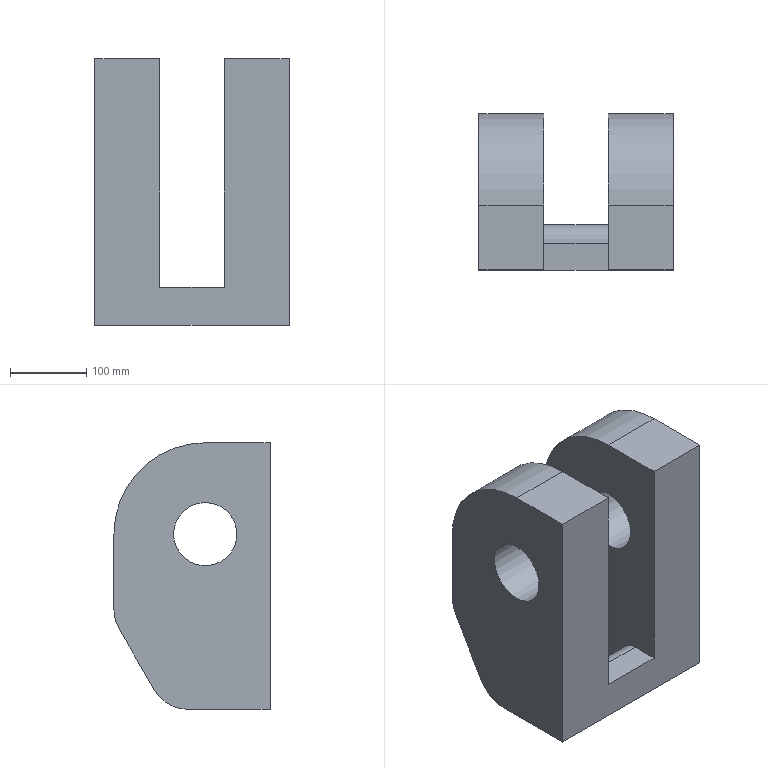Part | NX | features solid 2 | 1 solid | 22 faces | box 255 x 205 x 350 mm | volume 10284729 mm3 | plane 13 | cylinder 9 | commonest cylinder face diameters 100 x4 83 x2 240 x2 50 x1
STEP:
#1=CARTESIAN_POINT('',(-1395.,1008.453,-630.));
#2=VERTEX_POINT('',#1);
#3=CARTESIAN_POINT('',(-1395.,935.,-630.));
#4=VERTEX_POINT('',#3);
#5=CARTESIAN_POINT('',(-1395.,1105.,-630.));
#6=DIRECTION('',(0.,-1.,0.));
#7=VECTOR('',#6,1000.);
#8=LINE('',#5,#7);
#9=EDGE_CURVE('',#2,#4,#8,.T.);
#10=ORIENTED_EDGE('',*,*,#9,.F.);
#11=CARTESIAN_POINT('',(-1310.,1008.453,-630.));
#12=VERTEX_POINT('',#11);
#13=CARTESIAN_POINT('',(-1310.,1008.453,-630.));
#14=DIRECTION('',(1.,0.,0.));
#15=VECTOR('',#14,1000.);
#16=LINE('',#13,#15);
#17=EDGE_CURVE('',#2,#12,#16,.T.);
#18=ORIENTED_EDGE('',*,*,#17,.T.);
#19=CARTESIAN_POINT('',(-1310.,900.,-630.));
#20=VERTEX_POINT('',#19);
#21=CARTESIAN_POINT('',(-1310.,1105.,-630.));
#22=DIRECTION('',(0.,-1.,0.));
#23=VECTOR('',#22,1000.);
#24=LINE('',#21,#23);
#25=EDGE_CURVE('',#12,#20,#24,.T.);
#26=ORIENTED_EDGE('',*,*,#25,.T.);
#27=CARTESIAN_POINT('',(-1565.,900.,-630.));
#28=VERTEX_POINT('',#27);
#29=CARTESIAN_POINT('',(-1565.,900.,-630.));
#30=DIRECTION('',(1.,0.,0.));
#31=VECTOR('',#30,1000.);
#32=LINE('',#29,#31);
#33=EDGE_CURVE('',#28,#20,#32,.T.);
#34=ORIENTED_EDGE('',*,*,#33,.F.);
#35=CARTESIAN_POINT('',(-1565.,1008.453,-630.));
#36=VERTEX_POINT('',#35);
#37=CARTESIAN_POINT('',(-1565.,1105.,-630.));
#38=DIRECTION('',(0.,-1.,0.));
#39=VECTOR('',#38,1000.);
#40=LINE('',#37,#39);
#41=EDGE_CURVE('',#36,#28,#40,.T.);
#42=ORIENTED_EDGE('',*,*,#41,.F.);
#43=CARTESIAN_POINT('',(-1480.,1008.453,-630.));
#44=VERTEX_POINT('',#43);
#45=CARTESIAN_POINT('',(-1480.,1008.453,-630.));
#46=DIRECTION('',(1.,0.,0.));
#47=VECTOR('',#46,1000.);
#48=LINE('',#45,#47);
#49=EDGE_CURVE('',#36,#44,#48,.T.);
#50=ORIENTED_EDGE('',*,*,#49,.T.);
#51=CARTESIAN_POINT('',(-1480.,935.,-630.));
#52=VERTEX_POINT('',#51);
#53=CARTESIAN_POINT('',(-1480.,1105.,-630.));
#54=DIRECTION('',(0.,-1.,0.));
#55=VECTOR('',#54,1000.);
#56=LINE('',#53,#55);
#57=EDGE_CURVE('',#44,#52,#56,.T.);
#58=ORIENTED_EDGE('',*,*,#57,.T.);
#59=CARTESIAN_POINT('',(-1437.5,935.,-630.));
#60=DIRECTION('',(1.,0.,0.));
#61=VECTOR('',#60,1000.);
#62=LINE('',#59,#61);
#63=EDGE_CURVE('',#4,#52,#62,.F.);
#64=ORIENTED_EDGE('',*,*,#63,.F.);
#65=EDGE_LOOP('',(#10,#18,#26,#34,#42,#50,#58,#64));
#66=FACE_BOUND('',#65,.T.);
#67=CARTESIAN_POINT('',(-1565.,1105.,-630.));
#68=DIRECTION('',(0.,0.,1.));
#69=DIRECTION('',(0.,-1.,0.));
#70=AXIS2_PLACEMENT_3D('',#67,#68,#69);
#71=PLANE('',#70);
#72=ADVANCED_FACE('',(#66),#71,.F.);
#73=CARTESIAN_POINT('',(-1565.,985.,-280.));
#74=VERTEX_POINT('',#73);
#75=CARTESIAN_POINT('',(-1565.,900.,-280.));
#76=VERTEX_POINT('',#75);
#77=CARTESIAN_POINT('',(-1565.,1105.,-280.));
#78=DIRECTION('',(0.,-1.,0.));
#79=VECTOR('',#78,1000.);
#80=LINE('',#77,#79);
#81=EDGE_CURVE('',#74,#76,#80,.T.);
#82=ORIENTED_EDGE('',*,*,#81,.T.);
#83=CARTESIAN_POINT('',(-1480.,900.,-280.));
#84=VERTEX_POINT('',#83);
#85=CARTESIAN_POINT('',(-1565.,900.,-280.));
#86=DIRECTION('',(1.,0.,0.));
#87=VECTOR('',#86,1000.);
#88=LINE('',#85,#87);
#89=EDGE_CURVE('',#76,#84,#88,.T.);
#90=ORIENTED_EDGE('',*,*,#89,.T.);
#91=CARTESIAN_POINT('',(-1480.,985.,-280.));
#92=VERTEX_POINT('',#91);
#93=CARTESIAN_POINT('',(-1480.,1105.,-280.));
#94=DIRECTION('',(0.,1.,0.));
#95=VECTOR('',#94,1000.);
#96=LINE('',#93,#95);
#97=EDGE_CURVE('',#92,#84,#96,.F.);
#98=ORIENTED_EDGE('',*,*,#97,.F.);
#99=CARTESIAN_POINT('',(-1565.,985.,-280.));
#100=DIRECTION('',(-1.,0.,0.));
#101=VECTOR('',#100,1000.);
#102=LINE('',#99,#101);
#103=EDGE_CURVE('',#74,#92,#102,.F.);
#104=ORIENTED_EDGE('',*,*,#103,.F.);
#105=EDGE_LOOP('',(#82,#90,#98,#104));
#106=FACE_BOUND('',#105,.T.);
#107=CARTESIAN_POINT('',(-1565.,1105.,-280.));
#108=DIRECTION('',(0.,0.,1.));
#109=DIRECTION('',(0.,-1.,0.));
#110=AXIS2_PLACEMENT_3D('',#107,#108,#109);
#111=PLANE('',#110);
#112=ADVANCED_FACE('',(#106),#111,.T.);
#113=CARTESIAN_POINT('',(-1480.,1105.,-400.));
#114=VERTEX_POINT('',#113);
#115=CARTESIAN_POINT('',(-1480.,1105.,-499.378));
#116=VERTEX_POINT('',#115);
#117=CARTESIAN_POINT('',(-1480.,1105.,-280.));
#118=DIRECTION('',(0.,0.,-1.));
#119=VECTOR('',#118,1000.);
#120=LINE('',#117,#119);
#121=EDGE_CURVE('',#114,#116,#120,.T.);
#122=ORIENTED_EDGE('',*,*,#121,.T.);
#123=CARTESIAN_POINT('',(-1565.,1105.,-499.378));
#124=VERTEX_POINT('',#123);
#125=CARTESIAN_POINT('',(-1565.,1105.,-499.378));
#126=DIRECTION('',(-1.,0.,0.));
#127=VECTOR('',#126,1000.);
#128=LINE('',#125,#127);
#129=EDGE_CURVE('',#116,#124,#128,.T.);
#130=ORIENTED_EDGE('',*,*,#129,.T.);
#131=CARTESIAN_POINT('',(-1565.,1105.,-400.));
#132=VERTEX_POINT('',#131);
#133=CARTESIAN_POINT('',(-1565.,1105.,-280.));
#134=DIRECTION('',(0.,0.,-1.));
#135=VECTOR('',#134,1000.);
#136=LINE('',#133,#135);
#137=EDGE_CURVE('',#132,#124,#136,.T.);
#138=ORIENTED_EDGE('',*,*,#137,.F.);
#139=CARTESIAN_POINT('',(-1565.,1105.,-400.));
#140=DIRECTION('',(1.,0.,0.));
#141=VECTOR('',#140,1000.);
#142=LINE('',#139,#141);
#143=EDGE_CURVE('',#114,#132,#142,.F.);
#144=ORIENTED_EDGE('',*,*,#143,.F.);
#145=EDGE_LOOP('',(#122,#130,#138,#144));
#146=FACE_BOUND('',#145,.T.);
#147=CARTESIAN_POINT('',(-1565.,1105.,-280.));
#148=DIRECTION('',(0.,-1.,0.));
#149=DIRECTION('',(0.,0.,-1.));
#150=AXIS2_PLACEMENT_3D('',#147,#148,#149);
#151=PLANE('',#150);
#152=ADVANCED_FACE('',(#146),#151,.F.);
#153=CARTESIAN_POINT('',(-1310.,900.,-280.));
#154=VERTEX_POINT('',#153);
#155=CARTESIAN_POINT('',(-1310.,900.,-245.));
#156=DIRECTION('',(0.,0.,-1.));
#157=VECTOR('',#156,1000.);
#158=LINE('',#155,#157);
#159=EDGE_CURVE('',#154,#20,#158,.T.);
#160=ORIENTED_EDGE('',*,*,#159,.F.);
#161=CARTESIAN_POINT('',(-1395.,900.,-280.));
#162=VERTEX_POINT('',#161);
#163=CARTESIAN_POINT('',(-1395.,900.,-280.));
#164=DIRECTION('',(1.,0.,0.));
#165=VECTOR('',#164,1000.);
#166=LINE('',#163,#165);
#167=EDGE_CURVE('',#162,#154,#166,.T.);
#168=ORIENTED_EDGE('',*,*,#167,.F.);
#169=CARTESIAN_POINT('',(-1395.,900.,-580.));
#170=VERTEX_POINT('',#169);
#171=CARTESIAN_POINT('',(-1395.,900.,-245.));
#172=DIRECTION('',(0.,0.,-1.));
#173=VECTOR('',#172,1000.);
#174=LINE('',#171,#173);
#175=EDGE_CURVE('',#162,#170,#174,.T.);
#176=ORIENTED_EDGE('',*,*,#175,.T.);
#177=CARTESIAN_POINT('',(-1480.,900.,-580.));
#178=VERTEX_POINT('',#177);
#179=CARTESIAN_POINT('',(-1437.5,900.,-580.));
#180=DIRECTION('',(1.,0.,0.));
#181=VECTOR('',#180,1000.);
#182=LINE('',#179,#181);
#183=EDGE_CURVE('',#178,#170,#182,.T.);
#184=ORIENTED_EDGE('',*,*,#183,.F.);
#185=CARTESIAN_POINT('',(-1480.,900.,-245.));
#186=DIRECTION('',(0.,0.,-1.));
#187=VECTOR('',#186,1000.);
#188=LINE('',#185,#187);
#189=EDGE_CURVE('',#84,#178,#188,.T.);
#190=ORIENTED_EDGE('',*,*,#189,.F.);
#191=ORIENTED_EDGE('',*,*,#89,.F.);
#192=CARTESIAN_POINT('',(-1565.,900.,-245.));
#193=DIRECTION('',(0.,0.,-1.));
#194=VECTOR('',#193,1000.);
#195=LINE('',#192,#194);
#196=EDGE_CURVE('',#76,#28,#195,.T.);
#197=ORIENTED_EDGE('',*,*,#196,.T.);
#198=ORIENTED_EDGE('',*,*,#33,.T.);
#199=EDGE_LOOP('',(#160,#168,#176,#184,#190,#191,#197,#198));
#200=FACE_BOUND('',#199,.T.);
#201=CARTESIAN_POINT('',(-1565.,900.,-245.));
#202=DIRECTION('',(0.,-1.,0.));
#203=DIRECTION('',(0.,0.,-1.));
#204=AXIS2_PLACEMENT_3D('',#201,#202,#203);
#205=PLANE('',#204);
#206=ADVANCED_FACE('',(#200),#205,.T.);
#207=ORIENTED_EDGE('',*,*,#57,.F.);
#208=CARTESIAN_POINT('',(-1480.,1051.754,-605.));
#209=VERTEX_POINT('',#208);
#210=CARTESIAN_POINT('',(-1480.,1008.453,-580.));
#211=DIRECTION('',(-1.,0.,0.));
#212=DIRECTION('',(0.,0.,1.));
#213=AXIS2_PLACEMENT_3D('',#210,#211,#212);
#214=CIRCLE('',#213,50.);
#215=EDGE_CURVE('',#44,#209,#214,.F.);
#216=ORIENTED_EDGE('',*,*,#215,.T.);
#217=CARTESIAN_POINT('',(-1480.,1098.301,-524.378));
#218=VERTEX_POINT('',#217);
#219=CARTESIAN_POINT('',(-1480.,1174.286,-392.769));
#220=DIRECTION('',(0.,-0.5,-0.866));
#221=VECTOR('',#220,1000.);
#222=LINE('',#219,#221);
#223=EDGE_CURVE('',#218,#209,#222,.T.);
#224=ORIENTED_EDGE('',*,*,#223,.F.);
#225=CARTESIAN_POINT('',(-1480.,1055.,-499.378));
#226=DIRECTION('',(-1.,0.,0.));
#227=DIRECTION('',(0.,0.,1.));
#228=AXIS2_PLACEMENT_3D('',#225,#226,#227);
#229=CIRCLE('',#228,50.);
#230=EDGE_CURVE('',#218,#116,#229,.F.);
#231=ORIENTED_EDGE('',*,*,#230,.T.);
#232=ORIENTED_EDGE('',*,*,#121,.F.);
#233=CARTESIAN_POINT('',(-1480.,985.,-400.));
#234=DIRECTION('',(1.,0.,0.));
#235=DIRECTION('',(0.,0.,-1.));
#236=AXIS2_PLACEMENT_3D('',#233,#234,#235);
#237=CIRCLE('',#236,120.);
#238=EDGE_CURVE('',#92,#114,#237,.F.);
#239=ORIENTED_EDGE('',*,*,#238,.F.);
#240=ORIENTED_EDGE('',*,*,#97,.T.);
#241=ORIENTED_EDGE('',*,*,#189,.T.);
#242=CARTESIAN_POINT('',(-1480.,935.,-580.));
#243=VERTEX_POINT('',#242);
#244=CARTESIAN_POINT('',(-1480.,930.,-580.));
#245=DIRECTION('',(0.,-1.,0.));
#246=VECTOR('',#245,1000.);
#247=LINE('',#244,#246);
#248=EDGE_CURVE('',#243,#178,#247,.T.);
#249=ORIENTED_EDGE('',*,*,#248,.F.);
#250=CARTESIAN_POINT('',(-1480.,935.,-605.));
#251=DIRECTION('',(1.,0.,0.));
#252=DIRECTION('',(0.,0.,-1.));
#253=AXIS2_PLACEMENT_3D('',#250,#251,#252);
#254=CIRCLE('',#253,25.);
#255=EDGE_CURVE('',#52,#243,#254,.T.);
#256=ORIENTED_EDGE('',*,*,#255,.F.);
#257=EDGE_LOOP('',(#207,#216,#224,#231,#232,#239,#240,#241,#249,#256));
#258=FACE_BOUND('',#257,.T.);
#259=CARTESIAN_POINT('',(-1480.,985.,-441.5));
#260=VERTEX_POINT('',#259);
#261=CARTESIAN_POINT('',(-1480.,985.,-400.));
#262=DIRECTION('',(1.,0.,0.));
#263=DIRECTION('',(0.,0.,-1.));
#264=AXIS2_PLACEMENT_3D('',#261,#262,#263);
#265=CIRCLE('',#264,41.5);
#266=EDGE_CURVE('',#260,#260,#265,.T.);
#267=ORIENTED_EDGE('',*,*,#266,.F.);
#268=EDGE_LOOP('',(#267));
#269=FACE_BOUND('',#268,.T.);
#270=CARTESIAN_POINT('',(-1480.,1105.,-245.));
#271=DIRECTION('',(-1.,0.,0.));
#272=DIRECTION('',(0.,0.,-1.));
#273=AXIS2_PLACEMENT_3D('',#270,#271,#272);
#274=PLANE('',#273);
#275=ADVANCED_FACE('',(#258,#269),#274,.F.);
#276=CARTESIAN_POINT('',(-1565.,1098.301,-524.378));
#277=VERTEX_POINT('',#276);
#278=CARTESIAN_POINT('',(-1565.,1051.754,-605.));
#279=VERTEX_POINT('',#278);
#280=CARTESIAN_POINT('',(-1565.,1174.286,-392.769));
#281=DIRECTION('',(0.,-0.5,-0.866));
#282=VECTOR('',#281,1000.);
#283=LINE('',#280,#282);
#284=EDGE_CURVE('',#277,#279,#283,.T.);
#285=ORIENTED_EDGE('',*,*,#284,.T.);
#286=CARTESIAN_POINT('',(-1565.,1008.453,-580.));
#287=DIRECTION('',(-1.,0.,0.));
#288=DIRECTION('',(0.,0.,1.));
#289=AXIS2_PLACEMENT_3D('',#286,#287,#288);
#290=CIRCLE('',#289,50.);
#291=EDGE_CURVE('',#279,#36,#290,.T.);
#292=ORIENTED_EDGE('',*,*,#291,.T.);
#293=ORIENTED_EDGE('',*,*,#41,.T.);
#294=ORIENTED_EDGE('',*,*,#196,.F.);
#295=ORIENTED_EDGE('',*,*,#81,.F.);
#296=CARTESIAN_POINT('',(-1565.,985.,-400.));
#297=DIRECTION('',(1.,0.,0.));
#298=DIRECTION('',(0.,0.,-1.));
#299=AXIS2_PLACEMENT_3D('',#296,#297,#298);
#300=CIRCLE('',#299,120.);
#301=EDGE_CURVE('',#132,#74,#300,.T.);
#302=ORIENTED_EDGE('',*,*,#301,.F.);
#303=ORIENTED_EDGE('',*,*,#137,.T.);
#304=CARTESIAN_POINT('',(-1565.,1055.,-499.378));
#305=DIRECTION('',(-1.,0.,0.));
#306=DIRECTION('',(0.,0.,1.));
#307=AXIS2_PLACEMENT_3D('',#304,#305,#306);
#308=CIRCLE('',#307,50.);
#309=EDGE_CURVE('',#124,#277,#308,.T.);
#310=ORIENTED_EDGE('',*,*,#309,.T.);
#311=EDGE_LOOP('',(#285,#292,#293,#294,#295,#302,#303,#310));
#312=FACE_BOUND('',#311,.T.);
#313=CARTESIAN_POINT('',(-1565.,985.,-358.5));
#314=VERTEX_POINT('',#313);
#315=CARTESIAN_POINT('',(-1565.,985.,-400.));
#316=DIRECTION('',(-1.,0.,0.));
#317=DIRECTION('',(0.,0.,1.));
#318=AXIS2_PLACEMENT_3D('',#315,#316,#317);
#319=CIRCLE('',#318,41.5);
#320=EDGE_CURVE('',#314,#314,#319,.T.);
#321=ORIENTED_EDGE('',*,*,#320,.F.);
#322=EDGE_LOOP('',(#321));
#323=FACE_BOUND('',#322,.T.);
#324=CARTESIAN_POINT('',(-1565.,1105.,-245.));
#325=DIRECTION('',(-1.,0.,0.));
#326=DIRECTION('',(0.,0.,-1.));
#327=AXIS2_PLACEMENT_3D('',#324,#325,#326);
#328=PLANE('',#327);
#329=ADVANCED_FACE('',(#312,#323),#328,.T.);
#330=ORIENTED_EDGE('',*,*,#301,.T.);
#331=ORIENTED_EDGE('',*,*,#103,.T.);
#332=ORIENTED_EDGE('',*,*,#238,.T.);
#333=ORIENTED_EDGE('',*,*,#143,.T.);
#334=EDGE_LOOP('',(#330,#331,#332,#333));
#335=FACE_BOUND('',#334,.T.);
#336=CARTESIAN_POINT('',(-1565.,985.,-400.));
#337=DIRECTION('',(-1.,0.,0.));
#338=DIRECTION('',(0.,0.,-1.));
#339=AXIS2_PLACEMENT_3D('',#336,#337,#338);
#340=CYLINDRICAL_SURFACE('',#339,120.);
#341=ADVANCED_FACE('',(#335),#340,.T.);
#342=ORIENTED_EDGE('',*,*,#320,.T.);
#343=EDGE_LOOP('',(#342));
#344=FACE_BOUND('',#343,.T.);
#345=ORIENTED_EDGE('',*,*,#266,.T.);
#346=EDGE_LOOP('',(#345));
#347=FACE_BOUND('',#346,.T.);
#348=CARTESIAN_POINT('',(-1565.,985.,-400.));
#349=DIRECTION('',(1.,0.,0.));
#350=DIRECTION('',(0.,0.,1.));
#351=AXIS2_PLACEMENT_3D('',#348,#349,#350);
#352=CYLINDRICAL_SURFACE('',#351,41.5);
#353=ADVANCED_FACE('',(#344,#347),#352,.F.);
#354=ORIENTED_EDGE('',*,*,#248,.T.);
#355=ORIENTED_EDGE('',*,*,#183,.T.);
#356=CARTESIAN_POINT('',(-1395.,935.,-580.));
#357=VERTEX_POINT('',#356);
#358=CARTESIAN_POINT('',(-1395.,930.,-580.));
#359=DIRECTION('',(0.,1.,0.));
#360=VECTOR('',#359,1000.);
#361=LINE('',#358,#360);
#362=EDGE_CURVE('',#170,#357,#361,.T.);
#363=ORIENTED_EDGE('',*,*,#362,.T.);
#364=CARTESIAN_POINT('',(-1437.5,935.,-580.));
#365=DIRECTION('',(-1.,0.,0.));
#366=VECTOR('',#365,1000.);
#367=LINE('',#364,#366);
#368=EDGE_CURVE('',#243,#357,#367,.F.);
#369=ORIENTED_EDGE('',*,*,#368,.F.);
#370=EDGE_LOOP('',(#354,#355,#363,#369));
#371=FACE_BOUND('',#370,.T.);
#372=CARTESIAN_POINT('',(-1437.5,930.,-580.));
#373=DIRECTION('',(0.,0.,1.));
#374=DIRECTION('',(0.,1.,0.));
#375=AXIS2_PLACEMENT_3D('',#372,#373,#374);
#376=PLANE('',#375);
#377=ADVANCED_FACE('',(#371),#376,.T.);
#378=ORIENTED_EDGE('',*,*,#368,.T.);
#379=CARTESIAN_POINT('',(-1395.,935.,-605.));
#380=DIRECTION('',(-1.,0.,0.));
#381=DIRECTION('',(0.,0.,1.));
#382=AXIS2_PLACEMENT_3D('',#379,#380,#381);
#383=CIRCLE('',#382,25.);
#384=EDGE_CURVE('',#357,#4,#383,.T.);
#385=ORIENTED_EDGE('',*,*,#384,.T.);
#386=ORIENTED_EDGE('',*,*,#63,.T.);
#387=ORIENTED_EDGE('',*,*,#255,.T.);
#388=EDGE_LOOP('',(#378,#385,#386,#387));
#389=FACE_BOUND('',#388,.T.);
#390=CARTESIAN_POINT('',(-1437.5,935.,-605.));
#391=DIRECTION('',(-1.,0.,0.));
#392=DIRECTION('',(0.,0.,-1.));
#393=AXIS2_PLACEMENT_3D('',#390,#391,#392);
#394=CYLINDRICAL_SURFACE('',#393,25.);
#395=ADVANCED_FACE('',(#389),#394,.T.);
#396=CARTESIAN_POINT('',(-1395.,985.,-280.));
#397=VERTEX_POINT('',#396);
#398=CARTESIAN_POINT('',(-1395.,1105.,-280.));
#399=DIRECTION('',(0.,-1.,0.));
#400=VECTOR('',#399,1000.);
#401=LINE('',#398,#400);
#402=EDGE_CURVE('',#397,#162,#401,.T.);
#403=ORIENTED_EDGE('',*,*,#402,.T.);
#404=ORIENTED_EDGE('',*,*,#167,.T.);
#405=CARTESIAN_POINT('',(-1310.,985.,-280.));
#406=VERTEX_POINT('',#405);
#407=CARTESIAN_POINT('',(-1310.,1105.,-280.));
#408=DIRECTION('',(0.,1.,0.));
#409=VECTOR('',#408,1000.);
#410=LINE('',#407,#409);
#411=EDGE_CURVE('',#406,#154,#410,.F.);
#412=ORIENTED_EDGE('',*,*,#411,.F.);
#413=CARTESIAN_POINT('',(-1395.,985.,-280.));
#414=DIRECTION('',(-1.,0.,0.));
#415=VECTOR('',#414,1000.);
#416=LINE('',#413,#415);
#417=EDGE_CURVE('',#397,#406,#416,.F.);
#418=ORIENTED_EDGE('',*,*,#417,.F.);
#419=EDGE_LOOP('',(#403,#404,#412,#418));
#420=FACE_BOUND('',#419,.T.);
#421=CARTESIAN_POINT('',(-1395.,1105.,-280.));
#422=DIRECTION('',(0.,0.,1.));
#423=DIRECTION('',(0.,-1.,0.));
#424=AXIS2_PLACEMENT_3D('',#421,#422,#423);
#425=PLANE('',#424);
#426=ADVANCED_FACE('',(#420),#425,.T.);
#427=CARTESIAN_POINT('',(-1310.,1105.,-400.));
#428=VERTEX_POINT('',#427);
#429=CARTESIAN_POINT('',(-1310.,1105.,-499.378));
#430=VERTEX_POINT('',#429);
#431=CARTESIAN_POINT('',(-1310.,1105.,-280.));
#432=DIRECTION('',(0.,0.,-1.));
#433=VECTOR('',#432,1000.);
#434=LINE('',#431,#433);
#435=EDGE_CURVE('',#428,#430,#434,.T.);
#436=ORIENTED_EDGE('',*,*,#435,.T.);
#437=CARTESIAN_POINT('',(-1395.,1105.,-499.378));
#438=VERTEX_POINT('',#437);
#439=CARTESIAN_POINT('',(-1395.,1105.,-499.378));
#440=DIRECTION('',(-1.,0.,0.));
#441=VECTOR('',#440,1000.);
#442=LINE('',#439,#441);
#443=EDGE_CURVE('',#430,#438,#442,.T.);
#444=ORIENTED_EDGE('',*,*,#443,.T.);
#445=CARTESIAN_POINT('',(-1395.,1105.,-400.));
#446=VERTEX_POINT('',#445);
#447=CARTESIAN_POINT('',(-1395.,1105.,-280.));
#448=DIRECTION('',(0.,0.,-1.));
#449=VECTOR('',#448,1000.);
#450=LINE('',#447,#449);
#451=EDGE_CURVE('',#446,#438,#450,.T.);
#452=ORIENTED_EDGE('',*,*,#451,.F.);
#453=CARTESIAN_POINT('',(-1395.,1105.,-400.));
#454=DIRECTION('',(1.,0.,0.));
#455=VECTOR('',#454,1000.);
#456=LINE('',#453,#455);
#457=EDGE_CURVE('',#428,#446,#456,.F.);
#458=ORIENTED_EDGE('',*,*,#457,.F.);
#459=EDGE_LOOP('',(#436,#444,#452,#458));
#460=FACE_BOUND('',#459,.T.);
#461=CARTESIAN_POINT('',(-1395.,1105.,-280.));
#462=DIRECTION('',(0.,-1.,0.));
#463=DIRECTION('',(0.,0.,-1.));
#464=AXIS2_PLACEMENT_3D('',#461,#462,#463);
#465=PLANE('',#464);
#466=ADVANCED_FACE('',(#460),#465,.F.);
#467=ORIENTED_EDGE('',*,*,#25,.F.);
#468=CARTESIAN_POINT('',(-1310.,1051.754,-605.));
#469=VERTEX_POINT('',#468);
#470=CARTESIAN_POINT('',(-1310.,1008.453,-580.));
#471=DIRECTION('',(-1.,0.,0.));
#472=DIRECTION('',(0.,0.,1.));
#473=AXIS2_PLACEMENT_3D('',#470,#471,#472);
#474=CIRCLE('',#473,50.);
#475=EDGE_CURVE('',#12,#469,#474,.F.);
#476=ORIENTED_EDGE('',*,*,#475,.T.);
#477=CARTESIAN_POINT('',(-1310.,1098.301,-524.378));
#478=VERTEX_POINT('',#477);
#479=CARTESIAN_POINT('',(-1310.,1174.286,-392.769));
#480=DIRECTION('',(0.,-0.5,-0.866));
#481=VECTOR('',#480,1000.);
#482=LINE('',#479,#481);
#483=EDGE_CURVE('',#478,#469,#482,.T.);
#484=ORIENTED_EDGE('',*,*,#483,.F.);
#485=CARTESIAN_POINT('',(-1310.,1055.,-499.378));
#486=DIRECTION('',(-1.,0.,0.));
#487=DIRECTION('',(0.,0.,1.));
#488=AXIS2_PLACEMENT_3D('',#485,#486,#487);
#489=CIRCLE('',#488,50.);
#490=EDGE_CURVE('',#478,#430,#489,.F.);
#491=ORIENTED_EDGE('',*,*,#490,.T.);
#492=ORIENTED_EDGE('',*,*,#435,.F.);
#493=CARTESIAN_POINT('',(-1310.,985.,-400.));
#494=DIRECTION('',(1.,0.,0.));
#495=DIRECTION('',(0.,0.,-1.));
#496=AXIS2_PLACEMENT_3D('',#493,#494,#495);
#497=CIRCLE('',#496,120.);
#498=EDGE_CURVE('',#406,#428,#497,.F.);
#499=ORIENTED_EDGE('',*,*,#498,.F.);
#500=ORIENTED_EDGE('',*,*,#411,.T.);
#501=ORIENTED_EDGE('',*,*,#159,.T.);
#502=EDGE_LOOP('',(#467,#476,#484,#491,#492,#499,#500,#501));
#503=FACE_BOUND('',#502,.T.);
#504=CARTESIAN_POINT('',(-1310.,985.,-441.5));
#505=VERTEX_POINT('',#504);
#506=CARTESIAN_POINT('',(-1310.,985.,-400.));
#507=DIRECTION('',(1.,0.,0.));
#508=DIRECTION('',(0.,0.,-1.));
#509=AXIS2_PLACEMENT_3D('',#506,#507,#508);
#510=CIRCLE('',#509,41.5);
#511=EDGE_CURVE('',#505,#505,#510,.T.);
#512=ORIENTED_EDGE('',*,*,#511,.F.);
#513=EDGE_LOOP('',(#512));
#514=FACE_BOUND('',#513,.T.);
#515=CARTESIAN_POINT('',(-1310.,1105.,-245.));
#516=DIRECTION('',(-1.,0.,0.));
#517=DIRECTION('',(0.,0.,-1.));
#518=AXIS2_PLACEMENT_3D('',#515,#516,#517);
#519=PLANE('',#518);
#520=ADVANCED_FACE('',(#503,#514),#519,.F.);
#521=CARTESIAN_POINT('',(-1395.,1098.301,-524.378));
#522=VERTEX_POINT('',#521);
#523=CARTESIAN_POINT('',(-1395.,1051.754,-605.));
#524=VERTEX_POINT('',#523);
#525=CARTESIAN_POINT('',(-1395.,1174.286,-392.769));
#526=DIRECTION('',(0.,-0.5,-0.866));
#527=VECTOR('',#526,1000.);
#528=LINE('',#525,#527);
#529=EDGE_CURVE('',#522,#524,#528,.T.);
#530=ORIENTED_EDGE('',*,*,#529,.T.);
#531=CARTESIAN_POINT('',(-1395.,1008.453,-580.));
#532=DIRECTION('',(-1.,0.,0.));
#533=DIRECTION('',(0.,0.,1.));
#534=AXIS2_PLACEMENT_3D('',#531,#532,#533);
#535=CIRCLE('',#534,50.);
#536=EDGE_CURVE('',#524,#2,#535,.T.);
#537=ORIENTED_EDGE('',*,*,#536,.T.);
#538=ORIENTED_EDGE('',*,*,#9,.T.);
#539=ORIENTED_EDGE('',*,*,#384,.F.);
#540=ORIENTED_EDGE('',*,*,#362,.F.);
#541=ORIENTED_EDGE('',*,*,#175,.F.);
#542=ORIENTED_EDGE('',*,*,#402,.F.);
#543=CARTESIAN_POINT('',(-1395.,985.,-400.));
#544=DIRECTION('',(1.,0.,0.));
#545=DIRECTION('',(0.,0.,-1.));
#546=AXIS2_PLACEMENT_3D('',#543,#544,#545);
#547=CIRCLE('',#546,120.);
#548=EDGE_CURVE('',#446,#397,#547,.T.);
#549=ORIENTED_EDGE('',*,*,#548,.F.);
#550=ORIENTED_EDGE('',*,*,#451,.T.);
#551=CARTESIAN_POINT('',(-1395.,1055.,-499.378));
#552=DIRECTION('',(-1.,0.,0.));
#553=DIRECTION('',(0.,0.,1.));
#554=AXIS2_PLACEMENT_3D('',#551,#552,#553);
#555=CIRCLE('',#554,50.);
#556=EDGE_CURVE('',#438,#522,#555,.T.);
#557=ORIENTED_EDGE('',*,*,#556,.T.);
#558=EDGE_LOOP('',(#530,#537,#538,#539,#540,#541,#542,#549,#550,#557));
#559=FACE_BOUND('',#558,.T.);
#560=CARTESIAN_POINT('',(-1395.,985.,-358.5));
#561=VERTEX_POINT('',#560);
#562=CARTESIAN_POINT('',(-1395.,985.,-400.));
#563=DIRECTION('',(-1.,0.,0.));
#564=DIRECTION('',(0.,0.,1.));
#565=AXIS2_PLACEMENT_3D('',#562,#563,#564);
#566=CIRCLE('',#565,41.5);
#567=EDGE_CURVE('',#561,#561,#566,.T.);
#568=ORIENTED_EDGE('',*,*,#567,.F.);
#569=EDGE_LOOP('',(#568));
#570=FACE_BOUND('',#569,.T.);
#571=CARTESIAN_POINT('',(-1395.,1105.,-245.));
#572=DIRECTION('',(-1.,0.,0.));
#573=DIRECTION('',(0.,0.,-1.));
#574=AXIS2_PLACEMENT_3D('',#571,#572,#573);
#575=PLANE('',#574);
#576=ADVANCED_FACE('',(#559,#570),#575,.T.);
#577=ORIENTED_EDGE('',*,*,#548,.T.);
#578=ORIENTED_EDGE('',*,*,#417,.T.);
#579=ORIENTED_EDGE('',*,*,#498,.T.);
#580=ORIENTED_EDGE('',*,*,#457,.T.);
#581=EDGE_LOOP('',(#577,#578,#579,#580));
#582=FACE_BOUND('',#581,.T.);
#583=CARTESIAN_POINT('',(-1395.,985.,-400.));
#584=DIRECTION('',(-1.,0.,0.));
#585=DIRECTION('',(0.,0.,-1.));
#586=AXIS2_PLACEMENT_3D('',#583,#584,#585);
#587=CYLINDRICAL_SURFACE('',#586,120.);
#588=ADVANCED_FACE('',(#582),#587,.T.);
#589=ORIENTED_EDGE('',*,*,#567,.T.);
#590=EDGE_LOOP('',(#589));
#591=FACE_BOUND('',#590,.T.);
#592=ORIENTED_EDGE('',*,*,#511,.T.);
#593=EDGE_LOOP('',(#592));
#594=FACE_BOUND('',#593,.T.);
#595=CARTESIAN_POINT('',(-1395.,985.,-400.));
#596=DIRECTION('',(1.,0.,0.));
#597=DIRECTION('',(0.,0.,1.));
#598=AXIS2_PLACEMENT_3D('',#595,#596,#597);
#599=CYLINDRICAL_SURFACE('',#598,41.5);
#600=ADVANCED_FACE('',(#591,#594),#599,.F.);
#601=ORIENTED_EDGE('',*,*,#483,.T.);
#602=CARTESIAN_POINT('',(-1395.,1051.754,-605.));
#603=DIRECTION('',(-1.,0.,0.));
#604=VECTOR('',#603,1000.);
#605=LINE('',#602,#604);
#606=EDGE_CURVE('',#469,#524,#605,.T.);
#607=ORIENTED_EDGE('',*,*,#606,.T.);
#608=ORIENTED_EDGE('',*,*,#529,.F.);
#609=CARTESIAN_POINT('',(-1310.,1098.301,-524.378));
#610=DIRECTION('',(1.,0.,0.));
#611=VECTOR('',#610,1000.);
#612=LINE('',#609,#611);
#613=EDGE_CURVE('',#522,#478,#612,.T.);
#614=ORIENTED_EDGE('',*,*,#613,.T.);
#615=EDGE_LOOP('',(#601,#607,#608,#614));
#616=FACE_BOUND('',#615,.T.);
#617=CARTESIAN_POINT('',(-1565.,1048.868,-610.));
#618=DIRECTION('',(0.,-0.866,0.5));
#619=DIRECTION('',(0.,0.5,0.866));
#620=AXIS2_PLACEMENT_3D('',#617,#618,#619);
#621=PLANE('',#620);
#622=ADVANCED_FACE('',(#616),#621,.F.);
#623=ORIENTED_EDGE('',*,*,#223,.T.);
#624=CARTESIAN_POINT('',(-1565.,1051.754,-605.));
#625=DIRECTION('',(-1.,0.,0.));
#626=VECTOR('',#625,1000.);
#627=LINE('',#624,#626);
#628=EDGE_CURVE('',#209,#279,#627,.T.);
#629=ORIENTED_EDGE('',*,*,#628,.T.);
#630=ORIENTED_EDGE('',*,*,#284,.F.);
#631=CARTESIAN_POINT('',(-1480.,1098.301,-524.378));
#632=DIRECTION('',(1.,0.,0.));
#633=VECTOR('',#632,1000.);
#634=LINE('',#631,#633);
#635=EDGE_CURVE('',#277,#218,#634,.T.);
#636=ORIENTED_EDGE('',*,*,#635,.T.);
#637=EDGE_LOOP('',(#623,#629,#630,#636));
#638=FACE_BOUND('',#637,.T.);
#639=CARTESIAN_POINT('',(-1565.,1048.868,-610.));
#640=DIRECTION('',(0.,-0.866,0.5));
#641=DIRECTION('',(0.,0.5,0.866));
#642=AXIS2_PLACEMENT_3D('',#639,#640,#641);
#643=PLANE('',#642);
#644=ADVANCED_FACE('',(#638),#643,.F.);
#645=ORIENTED_EDGE('',*,*,#536,.F.);
#646=ORIENTED_EDGE('',*,*,#606,.F.);
#647=ORIENTED_EDGE('',*,*,#475,.F.);
#648=ORIENTED_EDGE('',*,*,#17,.F.);
#649=EDGE_LOOP('',(#645,#646,#647,#648));
#650=FACE_BOUND('',#649,.T.);
#651=CARTESIAN_POINT('',(-1565.,1008.453,-580.));
#652=DIRECTION('',(1.,0.,0.));
#653=DIRECTION('',(0.,-1.,0.));
#654=AXIS2_PLACEMENT_3D('',#651,#652,#653);
#655=CYLINDRICAL_SURFACE('',#654,50.);
#656=ADVANCED_FACE('',(#650),#655,.T.);
#657=ORIENTED_EDGE('',*,*,#291,.F.);
#658=ORIENTED_EDGE('',*,*,#628,.F.);
#659=ORIENTED_EDGE('',*,*,#215,.F.);
#660=ORIENTED_EDGE('',*,*,#49,.F.);
#661=EDGE_LOOP('',(#657,#658,#659,#660));
#662=FACE_BOUND('',#661,.T.);
#663=CARTESIAN_POINT('',(-1565.,1008.453,-580.));
#664=DIRECTION('',(1.,0.,0.));
#665=DIRECTION('',(0.,-1.,0.));
#666=AXIS2_PLACEMENT_3D('',#663,#664,#665);
#667=CYLINDRICAL_SURFACE('',#666,50.);
#668=ADVANCED_FACE('',(#662),#667,.T.);
#669=ORIENTED_EDGE('',*,*,#490,.F.);
#670=ORIENTED_EDGE('',*,*,#613,.F.);
#671=ORIENTED_EDGE('',*,*,#556,.F.);
#672=ORIENTED_EDGE('',*,*,#443,.F.);
#673=EDGE_LOOP('',(#669,#670,#671,#672));
#674=FACE_BOUND('',#673,.T.);
#675=CARTESIAN_POINT('',(-1395.,1055.,-499.378));
#676=DIRECTION('',(-1.,0.,0.));
#677=DIRECTION('',(0.,0.,1.));
#678=AXIS2_PLACEMENT_3D('',#675,#676,#677);
#679=CYLINDRICAL_SURFACE('',#678,50.);
#680=ADVANCED_FACE('',(#674),#679,.T.);
#681=ORIENTED_EDGE('',*,*,#230,.F.);
#682=ORIENTED_EDGE('',*,*,#635,.F.);
#683=ORIENTED_EDGE('',*,*,#309,.F.);
#684=ORIENTED_EDGE('',*,*,#129,.F.);
#685=EDGE_LOOP('',(#681,#682,#683,#684));
#686=FACE_BOUND('',#685,.T.);
#687=CARTESIAN_POINT('',(-1565.,1055.,-499.378));
#688=DIRECTION('',(-1.,0.,0.));
#689=DIRECTION('',(0.,0.,1.));
#690=AXIS2_PLACEMENT_3D('',#687,#688,#689);
#691=CYLINDRICAL_SURFACE('',#690,50.);
#692=ADVANCED_FACE('',(#686),#691,.T.);
#693=CLOSED_SHELL('',(#72,#112,#152,#206,#275,#329,#341,#353,#377,#395,#426,#466,#520,#576,#588,#600,#622,#644,#656,#668,#680,#692));
#694=MANIFOLD_SOLID_BREP('',#693);
#695=(LENGTH_UNIT()NAMED_UNIT(*)SI_UNIT(.MILLI.,.METRE.));
#696=UNCERTAINTY_MEASURE_WITH_UNIT(LENGTH_MEASURE(0.00001),#695,'','');
#697=(NAMED_UNIT(*)PLANE_ANGLE_UNIT()SI_UNIT($,.RADIAN.));
#698=(NAMED_UNIT(*)SI_UNIT($,.STERADIAN.)SOLID_ANGLE_UNIT());
#699=(GEOMETRIC_REPRESENTATION_CONTEXT(3)GLOBAL_UNCERTAINTY_ASSIGNED_CONTEXT((#696))GLOBAL_UNIT_ASSIGNED_CONTEXT((#695,#697,#698))REPRESENTATION_CONTEXT('',''));
#700=ADVANCED_BREP_SHAPE_REPRESENTATION('',(#694),#699);